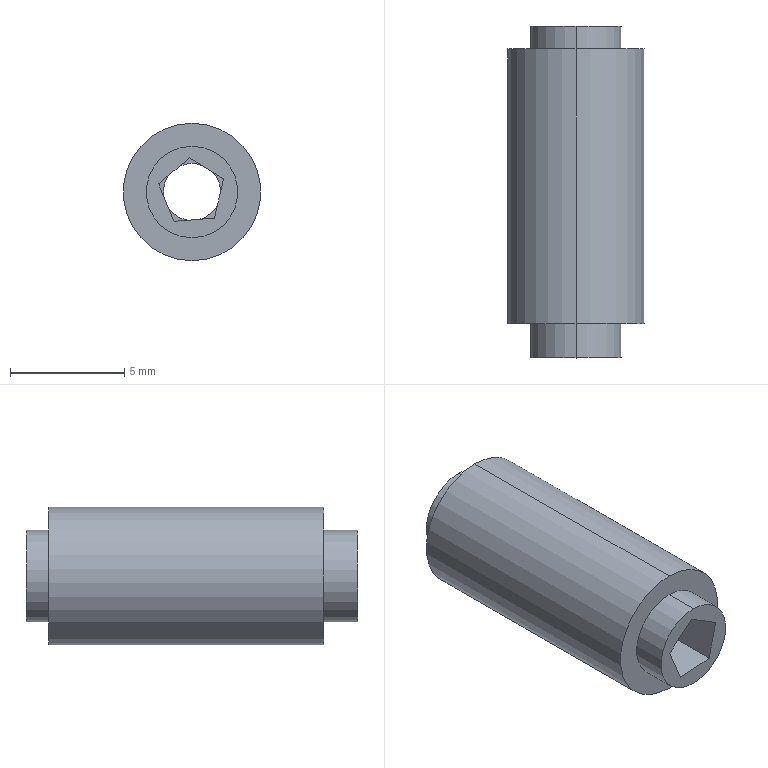Part | SolidWorks | features ICE 5, Extrusion 1 | 1 solid | 25 faces | box 6 x 14.5 x 6 mm | volume 291.486 mm3 | plane 15 | cylinder 10 | commonest cylinder face diameters 4 x4 2.5 x2 3 x2 6 x2
STEP:
#1=CARTESIAN_POINT('',(0.,4.5,-1.5));
#2=VERTEX_POINT('',#1);
#3=CARTESIAN_POINT('',(-0.7839,4.5,-1.279));
#4=VERTEX_POINT('',#3);
#5=CARTESIAN_POINT('',(0.,4.5,0.));
#6=DIRECTION('',(0.,1.,0.));
#7=DIRECTION('',(0.,0.,1.));
#8=AXIS2_PLACEMENT_3D('',#5,#6,#7);
#9=CIRCLE('',#8,1.5);
#10=EDGE_CURVE('',#2,#4,#9,.T.);
#11=ORIENTED_EDGE('',*,*,#10,.F.);
#12=CARTESIAN_POINT('',(0.,7.,-1.5));
#13=VERTEX_POINT('',#12);
#14=CARTESIAN_POINT('',(0.,4.5,-1.5));
#15=DIRECTION('',(0.,1.,0.));
#16=VECTOR('',#15,1000.);
#17=LINE('',#14,#16);
#18=EDGE_CURVE('',#2,#13,#17,.T.);
#19=ORIENTED_EDGE('',*,*,#18,.T.);
#20=CARTESIAN_POINT('',(0.,7.,1.5));
#21=VERTEX_POINT('',#20);
#22=CARTESIAN_POINT('',(0.,7.,0.));
#23=DIRECTION('',(0.,1.,0.));
#24=DIRECTION('',(0.,0.,1.));
#25=AXIS2_PLACEMENT_3D('',#22,#23,#24);
#26=CIRCLE('',#25,1.5);
#27=EDGE_CURVE('',#13,#21,#26,.T.);
#28=ORIENTED_EDGE('',*,*,#27,.T.);
#29=CARTESIAN_POINT('',(0.,4.5,1.5));
#30=VERTEX_POINT('',#29);
#31=CARTESIAN_POINT('',(0.,4.5,1.5));
#32=DIRECTION('',(0.,1.,0.));
#33=VECTOR('',#32,1000.);
#34=LINE('',#31,#33);
#35=EDGE_CURVE('',#30,#21,#34,.T.);
#36=ORIENTED_EDGE('',*,*,#35,.F.);
#37=CARTESIAN_POINT('',(-0.1176,4.5,1.495));
#38=VERTEX_POINT('',#37);
#39=CARTESIAN_POINT('',(0.,4.5,0.));
#40=DIRECTION('',(0.,1.,0.));
#41=DIRECTION('',(0.,0.,1.));
#42=AXIS2_PLACEMENT_3D('',#39,#40,#41);
#43=CIRCLE('',#42,1.5);
#44=EDGE_CURVE('',#38,#30,#43,.T.);
#45=ORIENTED_EDGE('',*,*,#44,.F.);
#46=CARTESIAN_POINT('',(-1.459,4.5,0.3503));
#47=VERTEX_POINT('',#46);
#48=CARTESIAN_POINT('',(0.,4.5,0.));
#49=DIRECTION('',(0.,1.,0.));
#50=DIRECTION('',(0.,0.,1.));
#51=AXIS2_PLACEMENT_3D('',#48,#49,#50);
#52=CIRCLE('',#51,1.5);
#53=EDGE_CURVE('',#47,#38,#52,.T.);
#54=ORIENTED_EDGE('',*,*,#53,.F.);
#55=CARTESIAN_POINT('',(0.,4.5,0.));
#56=DIRECTION('',(0.,1.,0.));
#57=DIRECTION('',(0.,0.,1.));
#58=AXIS2_PLACEMENT_3D('',#55,#56,#57);
#59=CIRCLE('',#58,1.5);
#60=EDGE_CURVE('',#4,#47,#59,.T.);
#61=ORIENTED_EDGE('',*,*,#60,.F.);
#62=EDGE_LOOP('',(#11,#19,#28,#36,#45,#54,#61));
#63=FACE_OUTER_BOUND('',#62,.T.);
#64=CARTESIAN_POINT('',(0.,4.5,0.));
#65=DIRECTION('',(0.,1.,0.));
#66=DIRECTION('',(0.,0.,1.));
#67=AXIS2_PLACEMENT_3D('',#64,#65,#66);
#68=CYLINDRICAL_SURFACE('',#67,1.5);
#69=ADVANCED_FACE('',(#63),#68,.F.);
#70=CARTESIAN_POINT('',(0.,7.,-1.25));
#71=VERTEX_POINT('',#70);
#72=CARTESIAN_POINT('',(0.,7.,1.25));
#73=VERTEX_POINT('',#72);
#74=CARTESIAN_POINT('',(0.,7.,0.));
#75=DIRECTION('',(0.,1.,0.));
#76=DIRECTION('',(0.,0.,1.));
#77=AXIS2_PLACEMENT_3D('',#74,#75,#76);
#78=CIRCLE('',#77,1.25);
#79=EDGE_CURVE('',#71,#73,#78,.T.);
#80=ORIENTED_EDGE('',*,*,#79,.F.);
#81=CARTESIAN_POINT('',(0.,13.,-1.25));
#82=VERTEX_POINT('',#81);
#83=CARTESIAN_POINT('',(0.,7.,-1.25));
#84=DIRECTION('',(0.,1.,0.));
#85=VECTOR('',#84,1000.);
#86=LINE('',#83,#85);
#87=EDGE_CURVE('',#71,#82,#86,.T.);
#88=ORIENTED_EDGE('',*,*,#87,.T.);
#89=CARTESIAN_POINT('',(0.,13.,1.25));
#90=VERTEX_POINT('',#89);
#91=CARTESIAN_POINT('',(0.,13.,0.));
#92=DIRECTION('',(0.,1.,0.));
#93=DIRECTION('',(0.,0.,1.));
#94=AXIS2_PLACEMENT_3D('',#91,#92,#93);
#95=CIRCLE('',#94,1.25);
#96=EDGE_CURVE('',#82,#90,#95,.T.);
#97=ORIENTED_EDGE('',*,*,#96,.T.);
#98=CARTESIAN_POINT('',(0.,7.,1.25));
#99=DIRECTION('',(0.,1.,0.));
#100=VECTOR('',#99,1000.);
#101=LINE('',#98,#100);
#102=EDGE_CURVE('',#73,#90,#101,.T.);
#103=ORIENTED_EDGE('',*,*,#102,.F.);
#104=EDGE_LOOP('',(#80,#88,#97,#103));
#105=FACE_OUTER_BOUND('',#104,.T.);
#106=CARTESIAN_POINT('',(0.,7.,0.));
#107=DIRECTION('',(0.,1.,0.));
#108=DIRECTION('',(0.,0.,1.));
#109=AXIS2_PLACEMENT_3D('',#106,#107,#108);
#110=CYLINDRICAL_SURFACE('',#109,1.25);
#111=ADVANCED_FACE('',(#105),#110,.F.);
#112=CARTESIAN_POINT('',(0.,-1.5,-2.));
#113=VERTEX_POINT('',#112);
#114=CARTESIAN_POINT('',(0.,-1.5,2.));
#115=VERTEX_POINT('',#114);
#116=CARTESIAN_POINT('',(0.,-1.5,0.));
#117=DIRECTION('',(0.,-1.,0.));
#118=DIRECTION('',(0.,0.,-1.));
#119=AXIS2_PLACEMENT_3D('',#116,#117,#118);
#120=CIRCLE('',#119,2.);
#121=EDGE_CURVE('',#113,#115,#120,.T.);
#122=ORIENTED_EDGE('',*,*,#121,.F.);
#123=CARTESIAN_POINT('',(0.,0.,-2.));
#124=VERTEX_POINT('',#123);
#125=CARTESIAN_POINT('',(0.,-1.5,-2.));
#126=DIRECTION('',(0.,1.,0.));
#127=VECTOR('',#126,1000.);
#128=LINE('',#125,#127);
#129=EDGE_CURVE('',#113,#124,#128,.T.);
#130=ORIENTED_EDGE('',*,*,#129,.T.);
#131=CARTESIAN_POINT('',(0.,0.,2.));
#132=VERTEX_POINT('',#131);
#133=CARTESIAN_POINT('',(0.,0.,0.));
#134=DIRECTION('',(0.,-1.,0.));
#135=DIRECTION('',(0.,0.,-1.));
#136=AXIS2_PLACEMENT_3D('',#133,#134,#135);
#137=CIRCLE('',#136,2.);
#138=EDGE_CURVE('',#124,#132,#137,.T.);
#139=ORIENTED_EDGE('',*,*,#138,.T.);
#140=CARTESIAN_POINT('',(0.,-1.5,2.));
#141=DIRECTION('',(0.,1.,0.));
#142=VECTOR('',#141,1000.);
#143=LINE('',#140,#142);
#144=EDGE_CURVE('',#115,#132,#143,.T.);
#145=ORIENTED_EDGE('',*,*,#144,.F.);
#146=EDGE_LOOP('',(#122,#130,#139,#145));
#147=FACE_OUTER_BOUND('',#146,.T.);
#148=CARTESIAN_POINT('',(0.,-1.5,0.));
#149=DIRECTION('',(0.,1.,0.));
#150=DIRECTION('',(0.,0.,1.));
#151=AXIS2_PLACEMENT_3D('',#148,#149,#150);
#152=CYLINDRICAL_SURFACE('',#151,2.);
#153=ADVANCED_FACE('',(#147),#152,.T.);
#154=CARTESIAN_POINT('',(0.,13.,2.));
#155=VERTEX_POINT('',#154);
#156=CARTESIAN_POINT('',(0.,13.,-2.));
#157=VERTEX_POINT('',#156);
#158=CARTESIAN_POINT('',(0.,13.,0.));
#159=DIRECTION('',(0.,1.,0.));
#160=DIRECTION('',(0.,0.,1.));
#161=AXIS2_PLACEMENT_3D('',#158,#159,#160);
#162=CIRCLE('',#161,2.);
#163=EDGE_CURVE('',#155,#157,#162,.T.);
#164=ORIENTED_EDGE('',*,*,#163,.F.);
#165=CARTESIAN_POINT('',(0.,12.,2.));
#166=VERTEX_POINT('',#165);
#167=CARTESIAN_POINT('',(0.,13.,2.));
#168=DIRECTION('',(0.,-1.,0.));
#169=VECTOR('',#168,1000.);
#170=LINE('',#167,#169);
#171=EDGE_CURVE('',#155,#166,#170,.T.);
#172=ORIENTED_EDGE('',*,*,#171,.T.);
#173=CARTESIAN_POINT('',(0.,12.,-2.));
#174=VERTEX_POINT('',#173);
#175=CARTESIAN_POINT('',(0.,12.,0.));
#176=DIRECTION('',(0.,1.,0.));
#177=DIRECTION('',(0.,0.,1.));
#178=AXIS2_PLACEMENT_3D('',#175,#176,#177);
#179=CIRCLE('',#178,2.);
#180=EDGE_CURVE('',#166,#174,#179,.T.);
#181=ORIENTED_EDGE('',*,*,#180,.T.);
#182=CARTESIAN_POINT('',(0.,13.,-2.));
#183=DIRECTION('',(0.,-1.,0.));
#184=VECTOR('',#183,1000.);
#185=LINE('',#182,#184);
#186=EDGE_CURVE('',#157,#174,#185,.T.);
#187=ORIENTED_EDGE('',*,*,#186,.F.);
#188=EDGE_LOOP('',(#164,#172,#181,#187));
#189=FACE_OUTER_BOUND('',#188,.T.);
#190=CARTESIAN_POINT('',(0.,13.,0.));
#191=DIRECTION('',(0.,-1.,0.));
#192=DIRECTION('',(0.,0.,-1.));
#193=AXIS2_PLACEMENT_3D('',#190,#191,#192);
#194=CYLINDRICAL_SURFACE('',#193,2.);
#195=ADVANCED_FACE('',(#189),#194,.T.);
#196=CARTESIAN_POINT('',(0.,12.,3.));
#197=VERTEX_POINT('',#196);
#198=CARTESIAN_POINT('',(0.,12.,-3.));
#199=VERTEX_POINT('',#198);
#200=CARTESIAN_POINT('',(0.,12.,0.));
#201=DIRECTION('',(0.,1.,0.));
#202=DIRECTION('',(0.,0.,1.));
#203=AXIS2_PLACEMENT_3D('',#200,#201,#202);
#204=CIRCLE('',#203,3.);
#205=EDGE_CURVE('',#197,#199,#204,.T.);
#206=ORIENTED_EDGE('',*,*,#205,.F.);
#207=CARTESIAN_POINT('',(0.,0.,3.));
#208=VERTEX_POINT('',#207);
#209=CARTESIAN_POINT('',(0.,12.,3.));
#210=DIRECTION('',(0.,-1.,0.));
#211=VECTOR('',#210,1000.);
#212=LINE('',#209,#211);
#213=EDGE_CURVE('',#197,#208,#212,.T.);
#214=ORIENTED_EDGE('',*,*,#213,.T.);
#215=CARTESIAN_POINT('',(0.,0.,-3.));
#216=VERTEX_POINT('',#215);
#217=CARTESIAN_POINT('',(0.,0.,0.));
#218=DIRECTION('',(0.,1.,0.));
#219=DIRECTION('',(0.,0.,1.));
#220=AXIS2_PLACEMENT_3D('',#217,#218,#219);
#221=CIRCLE('',#220,3.);
#222=EDGE_CURVE('',#208,#216,#221,.T.);
#223=ORIENTED_EDGE('',*,*,#222,.T.);
#224=CARTESIAN_POINT('',(0.,12.,-3.));
#225=DIRECTION('',(0.,-1.,0.));
#226=VECTOR('',#225,1000.);
#227=LINE('',#224,#226);
#228=EDGE_CURVE('',#199,#216,#227,.T.);
#229=ORIENTED_EDGE('',*,*,#228,.F.);
#230=EDGE_LOOP('',(#206,#214,#223,#229));
#231=FACE_OUTER_BOUND('',#230,.T.);
#232=CARTESIAN_POINT('',(0.,12.,0.));
#233=DIRECTION('',(0.,-1.,0.));
#234=DIRECTION('',(0.,0.,-1.));
#235=AXIS2_PLACEMENT_3D('',#232,#233,#234);
#236=CYLINDRICAL_SURFACE('',#235,3.);
#237=ADVANCED_FACE('',(#231),#236,.T.);
#238=CARTESIAN_POINT('',(0.9741,4.5,-1.141));
#239=VERTEX_POINT('',#238);
#240=CARTESIAN_POINT('',(0.,4.5,0.));
#241=DIRECTION('',(0.,1.,0.));
#242=DIRECTION('',(0.,0.,1.));
#243=AXIS2_PLACEMENT_3D('',#240,#241,#242);
#244=CIRCLE('',#243,1.5);
#245=EDGE_CURVE('',#239,#2,#244,.T.);
#246=ORIENTED_EDGE('',*,*,#245,.T.);
#247=ORIENTED_EDGE('',*,*,#10,.T.);
#248=CARTESIAN_POINT('',(-0.7839,4.5,-1.279));
#249=DIRECTION('',(0.9969,0.,0.07838));
#250=VECTOR('',#249,1000.);
#251=LINE('',#248,#250);
#252=EDGE_CURVE('',#4,#239,#251,.T.);
#253=ORIENTED_EDGE('',*,*,#252,.T.);
#254=EDGE_LOOP('',(#246,#247,#253));
#255=FACE_OUTER_BOUND('',#254,.T.);
#256=CARTESIAN_POINT('',(0.,4.5,0.));
#257=DIRECTION('',(0.,1.,0.));
#258=DIRECTION('',(0.,0.,1.));
#259=AXIS2_PLACEMENT_3D('',#256,#257,#258);
#260=PLANE('',#259);
#261=ADVANCED_FACE('',(#255),#260,.T.);
#262=ORIENTED_EDGE('',*,*,#60,.T.);
#263=CARTESIAN_POINT('',(-1.459,4.5,0.3503));
#264=DIRECTION('',(0.3826,0.,-0.9239));
#265=VECTOR('',#264,1000.);
#266=LINE('',#263,#265);
#267=EDGE_CURVE('',#47,#4,#266,.T.);
#268=ORIENTED_EDGE('',*,*,#267,.T.);
#269=EDGE_LOOP('',(#262,#268));
#270=FACE_OUTER_BOUND('',#269,.T.);
#271=CARTESIAN_POINT('',(0.,4.5,0.));
#272=DIRECTION('',(0.,1.,0.));
#273=DIRECTION('',(0.,0.,1.));
#274=AXIS2_PLACEMENT_3D('',#271,#272,#273);
#275=PLANE('',#274);
#276=ADVANCED_FACE('',(#270),#275,.T.);
#277=ORIENTED_EDGE('',*,*,#53,.T.);
#278=CARTESIAN_POINT('',(-0.1176,4.5,1.495));
#279=DIRECTION('',(-0.7605,0.,-0.6494));
#280=VECTOR('',#279,1000.);
#281=LINE('',#278,#280);
#282=EDGE_CURVE('',#38,#47,#281,.T.);
#283=ORIENTED_EDGE('',*,*,#282,.T.);
#284=EDGE_LOOP('',(#277,#283));
#285=FACE_OUTER_BOUND('',#284,.T.);
#286=CARTESIAN_POINT('',(0.,4.5,0.));
#287=DIRECTION('',(0.,1.,0.));
#288=DIRECTION('',(0.,0.,1.));
#289=AXIS2_PLACEMENT_3D('',#286,#287,#288);
#290=PLANE('',#289);
#291=ADVANCED_FACE('',(#285),#290,.T.);
#292=ORIENTED_EDGE('',*,*,#44,.T.);
#293=CARTESIAN_POINT('',(1.386,4.5,0.5739));
#294=VERTEX_POINT('',#293);
#295=CARTESIAN_POINT('',(0.,4.5,0.));
#296=DIRECTION('',(0.,1.,0.));
#297=DIRECTION('',(0.,0.,1.));
#298=AXIS2_PLACEMENT_3D('',#295,#296,#297);
#299=CIRCLE('',#298,1.5);
#300=EDGE_CURVE('',#30,#294,#299,.T.);
#301=ORIENTED_EDGE('',*,*,#300,.T.);
#302=CARTESIAN_POINT('',(1.386,4.5,0.5739));
#303=DIRECTION('',(-0.8526,0.,0.5226));
#304=VECTOR('',#303,1000.);
#305=LINE('',#302,#304);
#306=EDGE_CURVE('',#294,#38,#305,.T.);
#307=ORIENTED_EDGE('',*,*,#306,.T.);
#308=EDGE_LOOP('',(#292,#301,#307));
#309=FACE_OUTER_BOUND('',#308,.T.);
#310=CARTESIAN_POINT('',(0.,4.5,0.));
#311=DIRECTION('',(0.,1.,0.));
#312=DIRECTION('',(0.,0.,1.));
#313=AXIS2_PLACEMENT_3D('',#310,#311,#312);
#314=PLANE('',#313);
#315=ADVANCED_FACE('',(#309),#314,.T.);
#316=CARTESIAN_POINT('',(0.,4.5,0.));
#317=DIRECTION('',(0.,1.,0.));
#318=DIRECTION('',(0.,0.,1.));
#319=AXIS2_PLACEMENT_3D('',#316,#317,#318);
#320=CIRCLE('',#319,1.5);
#321=EDGE_CURVE('',#294,#239,#320,.T.);
#322=ORIENTED_EDGE('',*,*,#321,.T.);
#323=CARTESIAN_POINT('',(0.9741,4.5,-1.141));
#324=DIRECTION('',(0.2335,0.,0.9724));
#325=VECTOR('',#324,1000.);
#326=LINE('',#323,#325);
#327=EDGE_CURVE('',#239,#294,#326,.T.);
#328=ORIENTED_EDGE('',*,*,#327,.T.);
#329=EDGE_LOOP('',(#322,#328));
#330=FACE_OUTER_BOUND('',#329,.T.);
#331=CARTESIAN_POINT('',(0.,4.5,0.));
#332=DIRECTION('',(0.,1.,0.));
#333=DIRECTION('',(0.,0.,1.));
#334=AXIS2_PLACEMENT_3D('',#331,#332,#333);
#335=PLANE('',#334);
#336=ADVANCED_FACE('',(#330),#335,.T.);
#337=ORIENTED_EDGE('',*,*,#213,.F.);
#338=CARTESIAN_POINT('',(0.,12.,0.));
#339=DIRECTION('',(0.,1.,0.));
#340=DIRECTION('',(0.,0.,1.));
#341=AXIS2_PLACEMENT_3D('',#338,#339,#340);
#342=CIRCLE('',#341,3.);
#343=EDGE_CURVE('',#199,#197,#342,.T.);
#344=ORIENTED_EDGE('',*,*,#343,.F.);
#345=ORIENTED_EDGE('',*,*,#228,.T.);
#346=CARTESIAN_POINT('',(0.,0.,0.));
#347=DIRECTION('',(0.,1.,0.));
#348=DIRECTION('',(0.,0.,1.));
#349=AXIS2_PLACEMENT_3D('',#346,#347,#348);
#350=CIRCLE('',#349,3.);
#351=EDGE_CURVE('',#216,#208,#350,.T.);
#352=ORIENTED_EDGE('',*,*,#351,.T.);
#353=EDGE_LOOP('',(#337,#344,#345,#352));
#354=FACE_OUTER_BOUND('',#353,.T.);
#355=CARTESIAN_POINT('',(0.,12.,0.));
#356=DIRECTION('',(0.,-1.,0.));
#357=DIRECTION('',(0.,0.,-1.));
#358=AXIS2_PLACEMENT_3D('',#355,#356,#357);
#359=CYLINDRICAL_SURFACE('',#358,3.);
#360=ADVANCED_FACE('',(#354),#359,.T.);
#361=CARTESIAN_POINT('',(0.,12.,0.));
#362=DIRECTION('',(0.,1.,0.));
#363=DIRECTION('',(0.,0.,1.));
#364=AXIS2_PLACEMENT_3D('',#361,#362,#363);
#365=CIRCLE('',#364,2.);
#366=EDGE_CURVE('',#174,#166,#365,.T.);
#367=ORIENTED_EDGE('',*,*,#366,.F.);
#368=ORIENTED_EDGE('',*,*,#180,.F.);
#369=EDGE_LOOP('',(#367,#368));
#370=FACE_BOUND('',#369,.T.);
#371=ORIENTED_EDGE('',*,*,#343,.T.);
#372=ORIENTED_EDGE('',*,*,#205,.T.);
#373=EDGE_LOOP('',(#371,#372));
#374=FACE_OUTER_BOUND('',#373,.T.);
#375=CARTESIAN_POINT('',(0.,12.,0.));
#376=DIRECTION('',(0.,1.,0.));
#377=DIRECTION('',(0.,0.,1.));
#378=AXIS2_PLACEMENT_3D('',#375,#376,#377);
#379=PLANE('',#378);
#380=ADVANCED_FACE('',(#370,#374),#379,.T.);
#381=CARTESIAN_POINT('',(0.,0.,0.));
#382=DIRECTION('',(0.,-1.,0.));
#383=DIRECTION('',(0.,0.,-1.));
#384=AXIS2_PLACEMENT_3D('',#381,#382,#383);
#385=CIRCLE('',#384,2.);
#386=EDGE_CURVE('',#132,#124,#385,.T.);
#387=ORIENTED_EDGE('',*,*,#386,.F.);
#388=ORIENTED_EDGE('',*,*,#138,.F.);
#389=EDGE_LOOP('',(#387,#388));
#390=FACE_BOUND('',#389,.T.);
#391=ORIENTED_EDGE('',*,*,#351,.F.);
#392=ORIENTED_EDGE('',*,*,#222,.F.);
#393=EDGE_LOOP('',(#391,#392));
#394=FACE_OUTER_BOUND('',#393,.T.);
#395=CARTESIAN_POINT('',(0.,0.,0.));
#396=DIRECTION('',(0.,1.,0.));
#397=DIRECTION('',(0.,0.,1.));
#398=AXIS2_PLACEMENT_3D('',#395,#396,#397);
#399=PLANE('',#398);
#400=ADVANCED_FACE('',(#390,#394),#399,.F.);
#401=ORIENTED_EDGE('',*,*,#171,.F.);
#402=CARTESIAN_POINT('',(0.,13.,0.));
#403=DIRECTION('',(0.,1.,0.));
#404=DIRECTION('',(0.,0.,1.));
#405=AXIS2_PLACEMENT_3D('',#402,#403,#404);
#406=CIRCLE('',#405,2.);
#407=EDGE_CURVE('',#157,#155,#406,.T.);
#408=ORIENTED_EDGE('',*,*,#407,.F.);
#409=ORIENTED_EDGE('',*,*,#186,.T.);
#410=ORIENTED_EDGE('',*,*,#366,.T.);
#411=EDGE_LOOP('',(#401,#408,#409,#410));
#412=FACE_OUTER_BOUND('',#411,.T.);
#413=CARTESIAN_POINT('',(0.,13.,0.));
#414=DIRECTION('',(0.,-1.,0.));
#415=DIRECTION('',(0.,0.,-1.));
#416=AXIS2_PLACEMENT_3D('',#413,#414,#415);
#417=CYLINDRICAL_SURFACE('',#416,2.);
#418=ADVANCED_FACE('',(#412),#417,.T.);
#419=CARTESIAN_POINT('',(0.,13.,0.));
#420=DIRECTION('',(0.,1.,0.));
#421=DIRECTION('',(0.,0.,1.));
#422=AXIS2_PLACEMENT_3D('',#419,#420,#421);
#423=CIRCLE('',#422,1.25);
#424=EDGE_CURVE('',#90,#82,#423,.T.);
#425=ORIENTED_EDGE('',*,*,#424,.F.);
#426=ORIENTED_EDGE('',*,*,#96,.F.);
#427=EDGE_LOOP('',(#425,#426));
#428=FACE_BOUND('',#427,.T.);
#429=ORIENTED_EDGE('',*,*,#407,.T.);
#430=ORIENTED_EDGE('',*,*,#163,.T.);
#431=EDGE_LOOP('',(#429,#430));
#432=FACE_OUTER_BOUND('',#431,.T.);
#433=CARTESIAN_POINT('',(0.,13.,0.));
#434=DIRECTION('',(0.,1.,0.));
#435=DIRECTION('',(0.,0.,1.));
#436=AXIS2_PLACEMENT_3D('',#433,#434,#435);
#437=PLANE('',#436);
#438=ADVANCED_FACE('',(#428,#432),#437,.T.);
#439=ORIENTED_EDGE('',*,*,#129,.F.);
#440=CARTESIAN_POINT('',(0.,-1.5,0.));
#441=DIRECTION('',(0.,-1.,0.));
#442=DIRECTION('',(0.,0.,-1.));
#443=AXIS2_PLACEMENT_3D('',#440,#441,#442);
#444=CIRCLE('',#443,2.);
#445=EDGE_CURVE('',#115,#113,#444,.T.);
#446=ORIENTED_EDGE('',*,*,#445,.F.);
#447=ORIENTED_EDGE('',*,*,#144,.T.);
#448=ORIENTED_EDGE('',*,*,#386,.T.);
#449=EDGE_LOOP('',(#439,#446,#447,#448));
#450=FACE_OUTER_BOUND('',#449,.T.);
#451=CARTESIAN_POINT('',(0.,-1.5,0.));
#452=DIRECTION('',(0.,1.,0.));
#453=DIRECTION('',(0.,0.,1.));
#454=AXIS2_PLACEMENT_3D('',#451,#452,#453);
#455=CYLINDRICAL_SURFACE('',#454,2.);
#456=ADVANCED_FACE('',(#450),#455,.T.);
#457=CARTESIAN_POINT('',(-0.7839,-1.5,-1.279));
#458=VERTEX_POINT('',#457);
#459=CARTESIAN_POINT('',(0.9741,-1.5,-1.141));
#460=VERTEX_POINT('',#459);
#461=CARTESIAN_POINT('',(-0.7839,-1.5,-1.279));
#462=DIRECTION('',(0.9969,0.,0.07838));
#463=VECTOR('',#462,1000.);
#464=LINE('',#461,#463);
#465=EDGE_CURVE('',#458,#460,#464,.T.);
#466=ORIENTED_EDGE('',*,*,#465,.F.);
#467=CARTESIAN_POINT('',(-1.459,-1.5,0.3503));
#468=VERTEX_POINT('',#467);
#469=CARTESIAN_POINT('',(-1.459,-1.5,0.3503));
#470=DIRECTION('',(0.3826,0.,-0.9239));
#471=VECTOR('',#470,1000.);
#472=LINE('',#469,#471);
#473=EDGE_CURVE('',#468,#458,#472,.T.);
#474=ORIENTED_EDGE('',*,*,#473,.F.);
#475=CARTESIAN_POINT('',(-0.1176,-1.5,1.495));
#476=VERTEX_POINT('',#475);
#477=CARTESIAN_POINT('',(-0.1176,-1.5,1.495));
#478=DIRECTION('',(-0.7605,0.,-0.6494));
#479=VECTOR('',#478,1000.);
#480=LINE('',#477,#479);
#481=EDGE_CURVE('',#476,#468,#480,.T.);
#482=ORIENTED_EDGE('',*,*,#481,.F.);
#483=CARTESIAN_POINT('',(1.386,-1.5,0.5739));
#484=VERTEX_POINT('',#483);
#485=CARTESIAN_POINT('',(1.386,-1.5,0.5739));
#486=DIRECTION('',(-0.8526,0.,0.5226));
#487=VECTOR('',#486,1000.);
#488=LINE('',#485,#487);
#489=EDGE_CURVE('',#484,#476,#488,.T.);
#490=ORIENTED_EDGE('',*,*,#489,.F.);
#491=CARTESIAN_POINT('',(0.9741,-1.5,-1.141));
#492=DIRECTION('',(0.2335,0.,0.9724));
#493=VECTOR('',#492,1000.);
#494=LINE('',#491,#493);
#495=EDGE_CURVE('',#460,#484,#494,.T.);
#496=ORIENTED_EDGE('',*,*,#495,.F.);
#497=EDGE_LOOP('',(#466,#474,#482,#490,#496));
#498=FACE_BOUND('',#497,.T.);
#499=ORIENTED_EDGE('',*,*,#445,.T.);
#500=ORIENTED_EDGE('',*,*,#121,.T.);
#501=EDGE_LOOP('',(#499,#500));
#502=FACE_OUTER_BOUND('',#501,.T.);
#503=CARTESIAN_POINT('',(0.,-1.5,0.));
#504=DIRECTION('',(0.,-1.,0.));
#505=DIRECTION('',(0.,0.,-1.));
#506=AXIS2_PLACEMENT_3D('',#503,#504,#505);
#507=PLANE('',#506);
#508=ADVANCED_FACE('',(#498,#502),#507,.T.);
#509=ORIENTED_EDGE('',*,*,#87,.F.);
#510=CARTESIAN_POINT('',(0.,7.,0.));
#511=DIRECTION('',(0.,1.,0.));
#512=DIRECTION('',(0.,0.,1.));
#513=AXIS2_PLACEMENT_3D('',#510,#511,#512);
#514=CIRCLE('',#513,1.25);
#515=EDGE_CURVE('',#73,#71,#514,.T.);
#516=ORIENTED_EDGE('',*,*,#515,.F.);
#517=ORIENTED_EDGE('',*,*,#102,.T.);
#518=ORIENTED_EDGE('',*,*,#424,.T.);
#519=EDGE_LOOP('',(#509,#516,#517,#518));
#520=FACE_OUTER_BOUND('',#519,.T.);
#521=CARTESIAN_POINT('',(0.,7.,0.));
#522=DIRECTION('',(0.,1.,0.));
#523=DIRECTION('',(0.,0.,1.));
#524=AXIS2_PLACEMENT_3D('',#521,#522,#523);
#525=CYLINDRICAL_SURFACE('',#524,1.25);
#526=ADVANCED_FACE('',(#520),#525,.F.);
#527=ORIENTED_EDGE('',*,*,#18,.F.);
#528=ORIENTED_EDGE('',*,*,#245,.F.);
#529=ORIENTED_EDGE('',*,*,#321,.F.);
#530=ORIENTED_EDGE('',*,*,#300,.F.);
#531=ORIENTED_EDGE('',*,*,#35,.T.);
#532=CARTESIAN_POINT('',(0.,7.,0.));
#533=DIRECTION('',(0.,1.,0.));
#534=DIRECTION('',(0.,0.,1.));
#535=AXIS2_PLACEMENT_3D('',#532,#533,#534);
#536=CIRCLE('',#535,1.5);
#537=EDGE_CURVE('',#21,#13,#536,.T.);
#538=ORIENTED_EDGE('',*,*,#537,.T.);
#539=EDGE_LOOP('',(#527,#528,#529,#530,#531,#538));
#540=FACE_OUTER_BOUND('',#539,.T.);
#541=CARTESIAN_POINT('',(0.,4.5,0.));
#542=DIRECTION('',(0.,1.,0.));
#543=DIRECTION('',(0.,0.,1.));
#544=AXIS2_PLACEMENT_3D('',#541,#542,#543);
#545=CYLINDRICAL_SURFACE('',#544,1.5);
#546=ADVANCED_FACE('',(#540),#545,.F.);
#547=ORIENTED_EDGE('',*,*,#515,.T.);
#548=ORIENTED_EDGE('',*,*,#79,.T.);
#549=EDGE_LOOP('',(#547,#548));
#550=FACE_BOUND('',#549,.T.);
#551=ORIENTED_EDGE('',*,*,#537,.F.);
#552=ORIENTED_EDGE('',*,*,#27,.F.);
#553=EDGE_LOOP('',(#551,#552));
#554=FACE_OUTER_BOUND('',#553,.T.);
#555=CARTESIAN_POINT('',(0.,7.,0.));
#556=DIRECTION('',(0.,1.,0.));
#557=DIRECTION('',(0.,0.,1.));
#558=AXIS2_PLACEMENT_3D('',#555,#556,#557);
#559=PLANE('',#558);
#560=ADVANCED_FACE('',(#550,#554),#559,.F.);
#561=ORIENTED_EDGE('',*,*,#465,.T.);
#562=CARTESIAN_POINT('',(0.9741,4.5,-1.141));
#563=DIRECTION('',(0.,-1.,0.));
#564=VECTOR('',#563,1000.);
#565=LINE('',#562,#564);
#566=EDGE_CURVE('',#239,#460,#565,.T.);
#567=ORIENTED_EDGE('',*,*,#566,.F.);
#568=ORIENTED_EDGE('',*,*,#252,.F.);
#569=CARTESIAN_POINT('',(-0.7839,4.5,-1.279));
#570=DIRECTION('',(0.,-1.,0.));
#571=VECTOR('',#570,1000.);
#572=LINE('',#569,#571);
#573=EDGE_CURVE('',#4,#458,#572,.T.);
#574=ORIENTED_EDGE('',*,*,#573,.T.);
#575=EDGE_LOOP('',(#561,#567,#568,#574));
#576=FACE_OUTER_BOUND('',#575,.T.);
#577=CARTESIAN_POINT('',(-0.7839,4.5,-1.279));
#578=DIRECTION('',(0.07838,0.,-0.9969));
#579=DIRECTION('',(-0.9969,0.,-0.07838));
#580=AXIS2_PLACEMENT_3D('',#577,#578,#579);
#581=PLANE('',#580);
#582=ADVANCED_FACE('',(#576),#581,.F.);
#583=ORIENTED_EDGE('',*,*,#473,.T.);
#584=ORIENTED_EDGE('',*,*,#573,.F.);
#585=ORIENTED_EDGE('',*,*,#267,.F.);
#586=CARTESIAN_POINT('',(-1.459,4.5,0.3503));
#587=DIRECTION('',(0.,-1.,0.));
#588=VECTOR('',#587,1000.);
#589=LINE('',#586,#588);
#590=EDGE_CURVE('',#47,#468,#589,.T.);
#591=ORIENTED_EDGE('',*,*,#590,.T.);
#592=EDGE_LOOP('',(#583,#584,#585,#591));
#593=FACE_OUTER_BOUND('',#592,.T.);
#594=CARTESIAN_POINT('',(-1.459,4.5,0.3503));
#595=DIRECTION('',(-0.9239,0.,-0.3826));
#596=DIRECTION('',(-0.3826,0.,0.9239));
#597=AXIS2_PLACEMENT_3D('',#594,#595,#596);
#598=PLANE('',#597);
#599=ADVANCED_FACE('',(#593),#598,.F.);
#600=ORIENTED_EDGE('',*,*,#481,.T.);
#601=ORIENTED_EDGE('',*,*,#590,.F.);
#602=ORIENTED_EDGE('',*,*,#282,.F.);
#603=CARTESIAN_POINT('',(-0.1176,4.5,1.495));
#604=DIRECTION('',(0.,-1.,0.));
#605=VECTOR('',#604,1000.);
#606=LINE('',#603,#605);
#607=EDGE_CURVE('',#38,#476,#606,.T.);
#608=ORIENTED_EDGE('',*,*,#607,.T.);
#609=EDGE_LOOP('',(#600,#601,#602,#608));
#610=FACE_OUTER_BOUND('',#609,.T.);
#611=CARTESIAN_POINT('',(-0.1176,4.5,1.495));
#612=DIRECTION('',(-0.6494,0.,0.7605));
#613=DIRECTION('',(0.7605,0.,0.6494));
#614=AXIS2_PLACEMENT_3D('',#611,#612,#613);
#615=PLANE('',#614);
#616=ADVANCED_FACE('',(#610),#615,.F.);
#617=ORIENTED_EDGE('',*,*,#489,.T.);
#618=ORIENTED_EDGE('',*,*,#607,.F.);
#619=ORIENTED_EDGE('',*,*,#306,.F.);
#620=CARTESIAN_POINT('',(1.386,4.5,0.5739));
#621=DIRECTION('',(0.,-1.,0.));
#622=VECTOR('',#621,1000.);
#623=LINE('',#620,#622);
#624=EDGE_CURVE('',#294,#484,#623,.T.);
#625=ORIENTED_EDGE('',*,*,#624,.T.);
#626=EDGE_LOOP('',(#617,#618,#619,#625));
#627=FACE_OUTER_BOUND('',#626,.T.);
#628=CARTESIAN_POINT('',(1.386,4.5,0.5739));
#629=DIRECTION('',(0.5226,0.,0.8526));
#630=DIRECTION('',(0.8526,0.,-0.5226));
#631=AXIS2_PLACEMENT_3D('',#628,#629,#630);
#632=PLANE('',#631);
#633=ADVANCED_FACE('',(#627),#632,.F.);
#634=ORIENTED_EDGE('',*,*,#495,.T.);
#635=ORIENTED_EDGE('',*,*,#624,.F.);
#636=ORIENTED_EDGE('',*,*,#327,.F.);
#637=ORIENTED_EDGE('',*,*,#566,.T.);
#638=EDGE_LOOP('',(#634,#635,#636,#637));
#639=FACE_OUTER_BOUND('',#638,.T.);
#640=CARTESIAN_POINT('',(0.9741,4.5,-1.141));
#641=DIRECTION('',(0.9724,0.,-0.2335));
#642=DIRECTION('',(-0.2335,0.,-0.9724));
#643=AXIS2_PLACEMENT_3D('',#640,#641,#642);
#644=PLANE('',#643);
#645=ADVANCED_FACE('',(#639),#644,.F.);
#646=CLOSED_SHELL('',(#69,#111,#153,#195,#237,#261,#276,#291,#315,#336,#360,#380,#400,#418,#438,#456,#508,#526,#546,#560,#582,#599,#616,#633,#645));
#647=MANIFOLD_SOLID_BREP('',#646);
#648=CARTESIAN_POINT('',(0.,0.,0.));
#649=DIRECTION('',(0.,0.,1.));
#650=DIRECTION('',(1.,0.,0.));
#651=AXIS2_PLACEMENT_3D('',#648,#649,#650);
#652=(LENGTH_UNIT()NAMED_UNIT(*)SI_UNIT(.MILLI.,.METRE.));
#653=UNCERTAINTY_MEASURE_WITH_UNIT(LENGTH_MEASURE(0.00001),#652,'','');
#654=(NAMED_UNIT(*)PLANE_ANGLE_UNIT()SI_UNIT($,.RADIAN.));
#655=(NAMED_UNIT(*)SI_UNIT($,.STERADIAN.)SOLID_ANGLE_UNIT());
#656=(GEOMETRIC_REPRESENTATION_CONTEXT(3)GLOBAL_UNCERTAINTY_ASSIGNED_CONTEXT((#653))GLOBAL_UNIT_ASSIGNED_CONTEXT((#652,#654,#655))REPRESENTATION_CONTEXT('',''));
#657=ADVANCED_BREP_SHAPE_REPRESENTATION('',(#647,#651),#656);